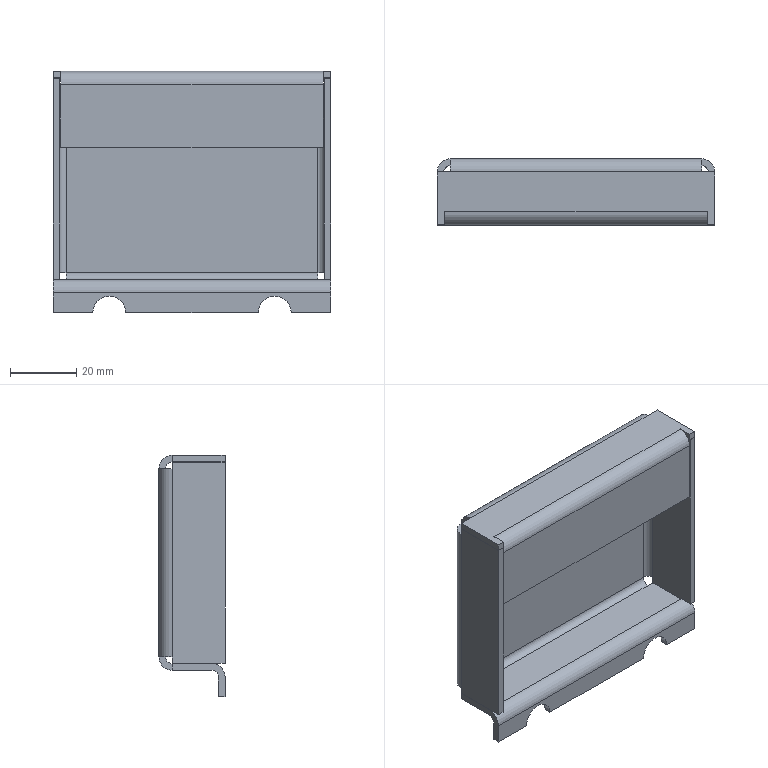Part | NX | features solid 2 | 1 solid | 66 faces | box 84 x 20 x 73 mm | volume 24541 mm3 | plane 52 | cylinder 14 | commonest cylinder face diameters 4 x6 8 x6 10 x2